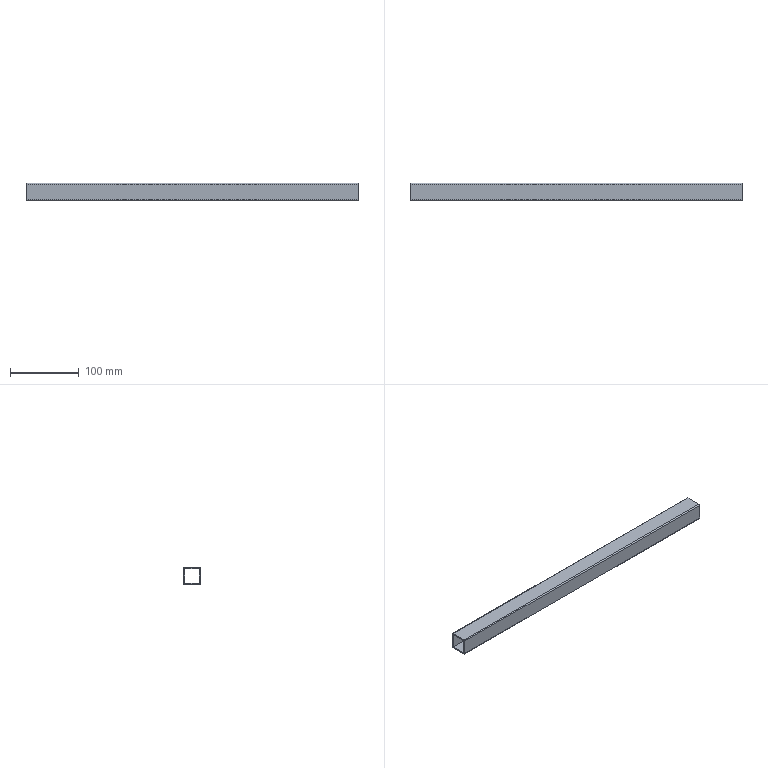Part | NX | features BREP 1 | 1 solid | 14 faces | box 482.6 x 25.4 x 25.4 mm | volume 84297 mm3 | plane 10 | cylinder 4 | commonest cylinder face diameters 3.175 x4
STEP:
#1=CARTESIAN_POINT('',(-241.3,12.7,-11.113));
#2=VERTEX_POINT('',#1);
#3=CARTESIAN_POINT('',(-241.3,12.7,11.113));
#4=VERTEX_POINT('',#3);
#5=CARTESIAN_POINT('',(-241.3,12.7,-11.113));
#6=DIRECTION('',(0.,0.,1.));
#7=VECTOR('',#6,1000.);
#8=LINE('',#5,#7);
#9=EDGE_CURVE('',#2,#4,#8,.T.);
#10=ORIENTED_EDGE('',*,*,#9,.F.);
#11=CARTESIAN_POINT('',(-241.3,11.113,-12.7));
#12=VERTEX_POINT('',#11);
#13=CARTESIAN_POINT('',(-241.3,11.113,-11.113));
#14=DIRECTION('',(-1.,0.,0.));
#15=DIRECTION('',(0.,1.,0.));
#16=AXIS2_PLACEMENT_3D('',#13,#14,#15);
#17=CIRCLE('',#16,1.587);
#18=EDGE_CURVE('',#2,#12,#17,.T.);
#19=ORIENTED_EDGE('',*,*,#18,.T.);
#20=CARTESIAN_POINT('',(-241.3,-11.113,-12.7));
#21=VERTEX_POINT('',#20);
#22=CARTESIAN_POINT('',(-241.3,-11.113,-12.7));
#23=DIRECTION('',(0.,1.,0.));
#24=VECTOR('',#23,1000.);
#25=LINE('',#22,#24);
#26=EDGE_CURVE('',#21,#12,#25,.T.);
#27=ORIENTED_EDGE('',*,*,#26,.F.);
#28=CARTESIAN_POINT('',(-241.3,-12.7,-11.113));
#29=VERTEX_POINT('',#28);
#30=CARTESIAN_POINT('',(-241.3,-11.113,-11.113));
#31=DIRECTION('',(-1.,0.,0.));
#32=DIRECTION('',(0.,0.,-1.));
#33=AXIS2_PLACEMENT_3D('',#30,#31,#32);
#34=CIRCLE('',#33,1.587);
#35=EDGE_CURVE('',#21,#29,#34,.T.);
#36=ORIENTED_EDGE('',*,*,#35,.T.);
#37=CARTESIAN_POINT('',(-241.3,-12.7,11.113));
#38=VERTEX_POINT('',#37);
#39=CARTESIAN_POINT('',(-241.3,-12.7,11.113));
#40=DIRECTION('',(0.,0.,-1.));
#41=VECTOR('',#40,1000.);
#42=LINE('',#39,#41);
#43=EDGE_CURVE('',#38,#29,#42,.T.);
#44=ORIENTED_EDGE('',*,*,#43,.F.);
#45=CARTESIAN_POINT('',(-241.3,-11.113,12.7));
#46=VERTEX_POINT('',#45);
#47=CARTESIAN_POINT('',(-241.3,-11.113,11.113));
#48=DIRECTION('',(-1.,0.,0.));
#49=DIRECTION('',(0.,-1.,0.));
#50=AXIS2_PLACEMENT_3D('',#47,#48,#49);
#51=CIRCLE('',#50,1.587);
#52=EDGE_CURVE('',#38,#46,#51,.T.);
#53=ORIENTED_EDGE('',*,*,#52,.T.);
#54=CARTESIAN_POINT('',(-241.3,11.113,12.7));
#55=VERTEX_POINT('',#54);
#56=CARTESIAN_POINT('',(-241.3,11.113,12.7));
#57=DIRECTION('',(0.,-1.,0.));
#58=VECTOR('',#57,1000.);
#59=LINE('',#56,#58);
#60=EDGE_CURVE('',#55,#46,#59,.T.);
#61=ORIENTED_EDGE('',*,*,#60,.F.);
#62=CARTESIAN_POINT('',(-241.3,11.113,11.113));
#63=DIRECTION('',(-1.,0.,0.));
#64=DIRECTION('',(0.,0.,1.));
#65=AXIS2_PLACEMENT_3D('',#62,#63,#64);
#66=CIRCLE('',#65,1.587);
#67=EDGE_CURVE('',#55,#4,#66,.T.);
#68=ORIENTED_EDGE('',*,*,#67,.T.);
#69=EDGE_LOOP('',(#10,#19,#27,#36,#44,#53,#61,#68));
#70=FACE_BOUND('',#69,.T.);
#71=CARTESIAN_POINT('',(-241.3,10.82,10.82));
#72=VERTEX_POINT('',#71);
#73=CARTESIAN_POINT('',(-241.3,10.82,-10.82));
#74=VERTEX_POINT('',#73);
#75=CARTESIAN_POINT('',(-241.3,10.82,10.82));
#76=DIRECTION('',(0.,0.,-1.));
#77=VECTOR('',#76,1000.);
#78=LINE('',#75,#77);
#79=EDGE_CURVE('',#72,#74,#78,.T.);
#80=ORIENTED_EDGE('',*,*,#79,.F.);
#81=CARTESIAN_POINT('',(-241.3,-10.82,10.82));
#82=VERTEX_POINT('',#81);
#83=CARTESIAN_POINT('',(-241.3,-10.82,10.82));
#84=DIRECTION('',(0.,1.,0.));
#85=VECTOR('',#84,1000.);
#86=LINE('',#83,#85);
#87=EDGE_CURVE('',#82,#72,#86,.T.);
#88=ORIENTED_EDGE('',*,*,#87,.F.);
#89=CARTESIAN_POINT('',(-241.3,-10.82,-10.82));
#90=VERTEX_POINT('',#89);
#91=CARTESIAN_POINT('',(-241.3,-10.82,-10.82));
#92=DIRECTION('',(0.,0.,1.));
#93=VECTOR('',#92,1000.);
#94=LINE('',#91,#93);
#95=EDGE_CURVE('',#90,#82,#94,.T.);
#96=ORIENTED_EDGE('',*,*,#95,.F.);
#97=CARTESIAN_POINT('',(-241.3,10.82,-10.82));
#98=DIRECTION('',(0.,-1.,0.));
#99=VECTOR('',#98,1000.);
#100=LINE('',#97,#99);
#101=EDGE_CURVE('',#74,#90,#100,.T.);
#102=ORIENTED_EDGE('',*,*,#101,.F.);
#103=EDGE_LOOP('',(#80,#88,#96,#102));
#104=FACE_BOUND('',#103,.T.);
#105=CARTESIAN_POINT('',(-241.3,0.,0.));
#106=DIRECTION('',(1.,0.,0.));
#107=DIRECTION('',(0.,1.,0.));
#108=AXIS2_PLACEMENT_3D('',#105,#106,#107);
#109=PLANE('',#108);
#110=ADVANCED_FACE('',(#70,#104),#109,.F.);
#111=CARTESIAN_POINT('',(241.3,-10.82,-10.82));
#112=VERTEX_POINT('',#111);
#113=CARTESIAN_POINT('',(-241.3,-10.82,-10.82));
#114=DIRECTION('',(1.,0.,0.));
#115=VECTOR('',#114,1000.);
#116=LINE('',#113,#115);
#117=EDGE_CURVE('',#90,#112,#116,.T.);
#118=ORIENTED_EDGE('',*,*,#117,.T.);
#119=CARTESIAN_POINT('',(241.3,10.82,-10.82));
#120=VERTEX_POINT('',#119);
#121=CARTESIAN_POINT('',(241.3,10.82,-10.82));
#122=DIRECTION('',(0.,-1.,0.));
#123=VECTOR('',#122,1000.);
#124=LINE('',#121,#123);
#125=EDGE_CURVE('',#120,#112,#124,.T.);
#126=ORIENTED_EDGE('',*,*,#125,.F.);
#127=CARTESIAN_POINT('',(-241.3,10.82,-10.82));
#128=DIRECTION('',(1.,0.,0.));
#129=VECTOR('',#128,1000.);
#130=LINE('',#127,#129);
#131=EDGE_CURVE('',#74,#120,#130,.T.);
#132=ORIENTED_EDGE('',*,*,#131,.F.);
#133=ORIENTED_EDGE('',*,*,#101,.T.);
#134=EDGE_LOOP('',(#118,#126,#132,#133));
#135=FACE_BOUND('',#134,.T.);
#136=CARTESIAN_POINT('',(-241.3,10.82,-10.82));
#137=DIRECTION('',(0.,0.,1.));
#138=DIRECTION('',(1.,0.,0.));
#139=AXIS2_PLACEMENT_3D('',#136,#137,#138);
#140=PLANE('',#139);
#141=ADVANCED_FACE('',(#135),#140,.T.);
#142=ORIENTED_EDGE('',*,*,#131,.T.);
#143=CARTESIAN_POINT('',(241.3,10.82,10.82));
#144=VERTEX_POINT('',#143);
#145=CARTESIAN_POINT('',(241.3,10.82,10.82));
#146=DIRECTION('',(0.,0.,-1.));
#147=VECTOR('',#146,1000.);
#148=LINE('',#145,#147);
#149=EDGE_CURVE('',#144,#120,#148,.T.);
#150=ORIENTED_EDGE('',*,*,#149,.F.);
#151=CARTESIAN_POINT('',(-241.3,10.82,10.82));
#152=DIRECTION('',(1.,0.,0.));
#153=VECTOR('',#152,1000.);
#154=LINE('',#151,#153);
#155=EDGE_CURVE('',#72,#144,#154,.T.);
#156=ORIENTED_EDGE('',*,*,#155,.F.);
#157=ORIENTED_EDGE('',*,*,#79,.T.);
#158=EDGE_LOOP('',(#142,#150,#156,#157));
#159=FACE_BOUND('',#158,.T.);
#160=CARTESIAN_POINT('',(-241.3,10.82,10.82));
#161=DIRECTION('',(0.,-1.,0.));
#162=DIRECTION('',(0.,0.,-1.));
#163=AXIS2_PLACEMENT_3D('',#160,#161,#162);
#164=PLANE('',#163);
#165=ADVANCED_FACE('',(#159),#164,.T.);
#166=ORIENTED_EDGE('',*,*,#155,.T.);
#167=CARTESIAN_POINT('',(241.3,-10.82,10.82));
#168=VERTEX_POINT('',#167);
#169=CARTESIAN_POINT('',(241.3,-10.82,10.82));
#170=DIRECTION('',(0.,1.,0.));
#171=VECTOR('',#170,1000.);
#172=LINE('',#169,#171);
#173=EDGE_CURVE('',#168,#144,#172,.T.);
#174=ORIENTED_EDGE('',*,*,#173,.F.);
#175=CARTESIAN_POINT('',(-241.3,-10.82,10.82));
#176=DIRECTION('',(1.,0.,0.));
#177=VECTOR('',#176,1000.);
#178=LINE('',#175,#177);
#179=EDGE_CURVE('',#82,#168,#178,.T.);
#180=ORIENTED_EDGE('',*,*,#179,.F.);
#181=ORIENTED_EDGE('',*,*,#87,.T.);
#182=EDGE_LOOP('',(#166,#174,#180,#181));
#183=FACE_BOUND('',#182,.T.);
#184=CARTESIAN_POINT('',(-241.3,-10.82,10.82));
#185=DIRECTION('',(0.,0.,-1.));
#186=DIRECTION('',(0.,-1.,0.));
#187=AXIS2_PLACEMENT_3D('',#184,#185,#186);
#188=PLANE('',#187);
#189=ADVANCED_FACE('',(#183),#188,.T.);
#190=ORIENTED_EDGE('',*,*,#179,.T.);
#191=CARTESIAN_POINT('',(241.3,-10.82,-10.82));
#192=DIRECTION('',(0.,0.,1.));
#193=VECTOR('',#192,1000.);
#194=LINE('',#191,#193);
#195=EDGE_CURVE('',#112,#168,#194,.T.);
#196=ORIENTED_EDGE('',*,*,#195,.F.);
#197=ORIENTED_EDGE('',*,*,#117,.F.);
#198=ORIENTED_EDGE('',*,*,#95,.T.);
#199=EDGE_LOOP('',(#190,#196,#197,#198));
#200=FACE_BOUND('',#199,.T.);
#201=CARTESIAN_POINT('',(-241.3,-10.82,-10.82));
#202=DIRECTION('',(0.,1.,0.));
#203=DIRECTION('',(1.,0.,0.));
#204=AXIS2_PLACEMENT_3D('',#201,#202,#203);
#205=PLANE('',#204);
#206=ADVANCED_FACE('',(#200),#205,.T.);
#207=CARTESIAN_POINT('',(241.3,11.113,12.7));
#208=VERTEX_POINT('',#207);
#209=CARTESIAN_POINT('',(241.3,-11.113,12.7));
#210=VERTEX_POINT('',#209);
#211=CARTESIAN_POINT('',(241.3,11.113,12.7));
#212=DIRECTION('',(0.,-1.,0.));
#213=VECTOR('',#212,1000.);
#214=LINE('',#211,#213);
#215=EDGE_CURVE('',#208,#210,#214,.T.);
#216=ORIENTED_EDGE('',*,*,#215,.T.);
#217=CARTESIAN_POINT('',(241.3,-12.7,11.113));
#218=VERTEX_POINT('',#217);
#219=CARTESIAN_POINT('',(241.3,-11.113,11.113));
#220=DIRECTION('',(1.,0.,0.));
#221=DIRECTION('',(0.,0.,1.));
#222=AXIS2_PLACEMENT_3D('',#219,#220,#221);
#223=CIRCLE('',#222,1.587);
#224=EDGE_CURVE('',#210,#218,#223,.T.);
#225=ORIENTED_EDGE('',*,*,#224,.T.);
#226=CARTESIAN_POINT('',(241.3,-12.7,-11.113));
#227=VERTEX_POINT('',#226);
#228=CARTESIAN_POINT('',(241.3,-12.7,11.113));
#229=DIRECTION('',(0.,0.,-1.));
#230=VECTOR('',#229,1000.);
#231=LINE('',#228,#230);
#232=EDGE_CURVE('',#218,#227,#231,.T.);
#233=ORIENTED_EDGE('',*,*,#232,.T.);
#234=CARTESIAN_POINT('',(241.3,-11.113,-12.7));
#235=VERTEX_POINT('',#234);
#236=CARTESIAN_POINT('',(241.3,-11.113,-11.113));
#237=DIRECTION('',(1.,0.,0.));
#238=DIRECTION('',(0.,-1.,0.));
#239=AXIS2_PLACEMENT_3D('',#236,#237,#238);
#240=CIRCLE('',#239,1.587);
#241=EDGE_CURVE('',#227,#235,#240,.T.);
#242=ORIENTED_EDGE('',*,*,#241,.T.);
#243=CARTESIAN_POINT('',(241.3,11.113,-12.7));
#244=VERTEX_POINT('',#243);
#245=CARTESIAN_POINT('',(241.3,-11.113,-12.7));
#246=DIRECTION('',(0.,1.,0.));
#247=VECTOR('',#246,1000.);
#248=LINE('',#245,#247);
#249=EDGE_CURVE('',#235,#244,#248,.T.);
#250=ORIENTED_EDGE('',*,*,#249,.T.);
#251=CARTESIAN_POINT('',(241.3,12.7,-11.113));
#252=VERTEX_POINT('',#251);
#253=CARTESIAN_POINT('',(241.3,11.113,-11.113));
#254=DIRECTION('',(1.,0.,0.));
#255=DIRECTION('',(0.,0.,-1.));
#256=AXIS2_PLACEMENT_3D('',#253,#254,#255);
#257=CIRCLE('',#256,1.587);
#258=EDGE_CURVE('',#244,#252,#257,.T.);
#259=ORIENTED_EDGE('',*,*,#258,.T.);
#260=CARTESIAN_POINT('',(241.3,12.7,11.113));
#261=VERTEX_POINT('',#260);
#262=CARTESIAN_POINT('',(241.3,12.7,-11.113));
#263=DIRECTION('',(0.,0.,1.));
#264=VECTOR('',#263,1000.);
#265=LINE('',#262,#264);
#266=EDGE_CURVE('',#252,#261,#265,.T.);
#267=ORIENTED_EDGE('',*,*,#266,.T.);
#268=CARTESIAN_POINT('',(241.3,11.113,11.113));
#269=DIRECTION('',(1.,0.,0.));
#270=DIRECTION('',(0.,1.,0.));
#271=AXIS2_PLACEMENT_3D('',#268,#269,#270);
#272=CIRCLE('',#271,1.587);
#273=EDGE_CURVE('',#261,#208,#272,.T.);
#274=ORIENTED_EDGE('',*,*,#273,.T.);
#275=EDGE_LOOP('',(#216,#225,#233,#242,#250,#259,#267,#274));
#276=FACE_BOUND('',#275,.T.);
#277=ORIENTED_EDGE('',*,*,#195,.T.);
#278=ORIENTED_EDGE('',*,*,#173,.T.);
#279=ORIENTED_EDGE('',*,*,#149,.T.);
#280=ORIENTED_EDGE('',*,*,#125,.T.);
#281=EDGE_LOOP('',(#277,#278,#279,#280));
#282=FACE_BOUND('',#281,.T.);
#283=CARTESIAN_POINT('',(241.3,0.,0.));
#284=DIRECTION('',(1.,0.,0.));
#285=DIRECTION('',(0.,1.,0.));
#286=AXIS2_PLACEMENT_3D('',#283,#284,#285);
#287=PLANE('',#286);
#288=ADVANCED_FACE('',(#276,#282),#287,.T.);
#289=ORIENTED_EDGE('',*,*,#273,.F.);
#290=CARTESIAN_POINT('',(241.3,12.7,11.113));
#291=DIRECTION('',(-1.,0.,0.));
#292=VECTOR('',#291,1000.);
#293=LINE('',#290,#292);
#294=EDGE_CURVE('',#261,#4,#293,.T.);
#295=ORIENTED_EDGE('',*,*,#294,.T.);
#296=ORIENTED_EDGE('',*,*,#67,.F.);
#297=CARTESIAN_POINT('',(241.3,11.113,12.7));
#298=DIRECTION('',(-1.,0.,0.));
#299=VECTOR('',#298,1000.);
#300=LINE('',#297,#299);
#301=EDGE_CURVE('',#208,#55,#300,.T.);
#302=ORIENTED_EDGE('',*,*,#301,.F.);
#303=EDGE_LOOP('',(#289,#295,#296,#302));
#304=FACE_BOUND('',#303,.T.);
#305=CARTESIAN_POINT('',(242.057,11.113,11.113));
#306=DIRECTION('',(-1.,0.,0.));
#307=DIRECTION('',(0.,0.,1.));
#308=AXIS2_PLACEMENT_3D('',#305,#306,#307);
#309=CYLINDRICAL_SURFACE('',#308,1.587);
#310=ADVANCED_FACE('',(#304),#309,.T.);
#311=ORIENTED_EDGE('',*,*,#60,.T.);
#312=CARTESIAN_POINT('',(241.3,-11.113,12.7));
#313=DIRECTION('',(-1.,0.,0.));
#314=VECTOR('',#313,1000.);
#315=LINE('',#312,#314);
#316=EDGE_CURVE('',#210,#46,#315,.T.);
#317=ORIENTED_EDGE('',*,*,#316,.F.);
#318=ORIENTED_EDGE('',*,*,#215,.F.);
#319=ORIENTED_EDGE('',*,*,#301,.T.);
#320=EDGE_LOOP('',(#311,#317,#318,#319));
#321=FACE_BOUND('',#320,.T.);
#322=CARTESIAN_POINT('',(-241.3,12.7,12.7));
#323=DIRECTION('',(0.,0.,1.));
#324=DIRECTION('',(1.,0.,0.));
#325=AXIS2_PLACEMENT_3D('',#322,#323,#324);
#326=PLANE('',#325);
#327=ADVANCED_FACE('',(#321),#326,.T.);
#328=ORIENTED_EDGE('',*,*,#224,.F.);
#329=ORIENTED_EDGE('',*,*,#316,.T.);
#330=ORIENTED_EDGE('',*,*,#52,.F.);
#331=CARTESIAN_POINT('',(241.3,-12.7,11.113));
#332=DIRECTION('',(-1.,0.,0.));
#333=VECTOR('',#332,1000.);
#334=LINE('',#331,#333);
#335=EDGE_CURVE('',#218,#38,#334,.T.);
#336=ORIENTED_EDGE('',*,*,#335,.F.);
#337=EDGE_LOOP('',(#328,#329,#330,#336));
#338=FACE_BOUND('',#337,.T.);
#339=CARTESIAN_POINT('',(242.057,-11.113,11.113));
#340=DIRECTION('',(-1.,0.,0.));
#341=DIRECTION('',(0.,-1.,0.));
#342=AXIS2_PLACEMENT_3D('',#339,#340,#341);
#343=CYLINDRICAL_SURFACE('',#342,1.587);
#344=ADVANCED_FACE('',(#338),#343,.T.);
#345=ORIENTED_EDGE('',*,*,#43,.T.);
#346=CARTESIAN_POINT('',(241.3,-12.7,-11.113));
#347=DIRECTION('',(-1.,0.,0.));
#348=VECTOR('',#347,1000.);
#349=LINE('',#346,#348);
#350=EDGE_CURVE('',#227,#29,#349,.T.);
#351=ORIENTED_EDGE('',*,*,#350,.F.);
#352=ORIENTED_EDGE('',*,*,#232,.F.);
#353=ORIENTED_EDGE('',*,*,#335,.T.);
#354=EDGE_LOOP('',(#345,#351,#352,#353));
#355=FACE_BOUND('',#354,.T.);
#356=CARTESIAN_POINT('',(-241.3,-12.7,12.7));
#357=DIRECTION('',(0.,-1.,0.));
#358=DIRECTION('',(0.,0.,-1.));
#359=AXIS2_PLACEMENT_3D('',#356,#357,#358);
#360=PLANE('',#359);
#361=ADVANCED_FACE('',(#355),#360,.T.);
#362=ORIENTED_EDGE('',*,*,#241,.F.);
#363=ORIENTED_EDGE('',*,*,#350,.T.);
#364=ORIENTED_EDGE('',*,*,#35,.F.);
#365=CARTESIAN_POINT('',(241.3,-11.113,-12.7));
#366=DIRECTION('',(-1.,0.,0.));
#367=VECTOR('',#366,1000.);
#368=LINE('',#365,#367);
#369=EDGE_CURVE('',#235,#21,#368,.T.);
#370=ORIENTED_EDGE('',*,*,#369,.F.);
#371=EDGE_LOOP('',(#362,#363,#364,#370));
#372=FACE_BOUND('',#371,.T.);
#373=CARTESIAN_POINT('',(242.057,-11.113,-11.113));
#374=DIRECTION('',(-1.,0.,0.));
#375=DIRECTION('',(0.,0.,-1.));
#376=AXIS2_PLACEMENT_3D('',#373,#374,#375);
#377=CYLINDRICAL_SURFACE('',#376,1.587);
#378=ADVANCED_FACE('',(#372),#377,.T.);
#379=ORIENTED_EDGE('',*,*,#249,.F.);
#380=ORIENTED_EDGE('',*,*,#369,.T.);
#381=ORIENTED_EDGE('',*,*,#26,.T.);
#382=CARTESIAN_POINT('',(241.3,11.113,-12.7));
#383=DIRECTION('',(-1.,0.,0.));
#384=VECTOR('',#383,1000.);
#385=LINE('',#382,#384);
#386=EDGE_CURVE('',#244,#12,#385,.T.);
#387=ORIENTED_EDGE('',*,*,#386,.F.);
#388=EDGE_LOOP('',(#379,#380,#381,#387));
#389=FACE_BOUND('',#388,.T.);
#390=CARTESIAN_POINT('',(-241.3,-12.7,-12.7));
#391=DIRECTION('',(0.,0.,-1.));
#392=DIRECTION('',(0.,-1.,0.));
#393=AXIS2_PLACEMENT_3D('',#390,#391,#392);
#394=PLANE('',#393);
#395=ADVANCED_FACE('',(#389),#394,.T.);
#396=ORIENTED_EDGE('',*,*,#258,.F.);
#397=ORIENTED_EDGE('',*,*,#386,.T.);
#398=ORIENTED_EDGE('',*,*,#18,.F.);
#399=CARTESIAN_POINT('',(241.3,12.7,-11.113));
#400=DIRECTION('',(-1.,0.,0.));
#401=VECTOR('',#400,1000.);
#402=LINE('',#399,#401);
#403=EDGE_CURVE('',#252,#2,#402,.T.);
#404=ORIENTED_EDGE('',*,*,#403,.F.);
#405=EDGE_LOOP('',(#396,#397,#398,#404));
#406=FACE_BOUND('',#405,.T.);
#407=CARTESIAN_POINT('',(242.057,11.113,-11.113));
#408=DIRECTION('',(-1.,0.,0.));
#409=DIRECTION('',(0.,1.,0.));
#410=AXIS2_PLACEMENT_3D('',#407,#408,#409);
#411=CYLINDRICAL_SURFACE('',#410,1.587);
#412=ADVANCED_FACE('',(#406),#411,.T.);
#413=ORIENTED_EDGE('',*,*,#266,.F.);
#414=ORIENTED_EDGE('',*,*,#403,.T.);
#415=ORIENTED_EDGE('',*,*,#9,.T.);
#416=ORIENTED_EDGE('',*,*,#294,.F.);
#417=EDGE_LOOP('',(#413,#414,#415,#416));
#418=FACE_BOUND('',#417,.T.);
#419=CARTESIAN_POINT('',(-241.3,12.7,-12.7));
#420=DIRECTION('',(0.,1.,0.));
#421=DIRECTION('',(1.,0.,0.));
#422=AXIS2_PLACEMENT_3D('',#419,#420,#421);
#423=PLANE('',#422);
#424=ADVANCED_FACE('',(#418),#423,.T.);
#425=CLOSED_SHELL('',(#110,#141,#165,#189,#206,#288,#310,#327,#344,#361,#378,#395,#412,#424));
#426=MANIFOLD_SOLID_BREP('',#425);
#427=(LENGTH_UNIT()NAMED_UNIT(*)SI_UNIT(.MILLI.,.METRE.));
#428=UNCERTAINTY_MEASURE_WITH_UNIT(LENGTH_MEASURE(0.00001),#427,'','');
#429=(NAMED_UNIT(*)PLANE_ANGLE_UNIT()SI_UNIT($,.RADIAN.));
#430=(NAMED_UNIT(*)SI_UNIT($,.STERADIAN.)SOLID_ANGLE_UNIT());
#431=(GEOMETRIC_REPRESENTATION_CONTEXT(3)GLOBAL_UNCERTAINTY_ASSIGNED_CONTEXT((#428))GLOBAL_UNIT_ASSIGNED_CONTEXT((#427,#429,#430))REPRESENTATION_CONTEXT('',''));
#432=ADVANCED_BREP_SHAPE_REPRESENTATION('',(#426),#431);